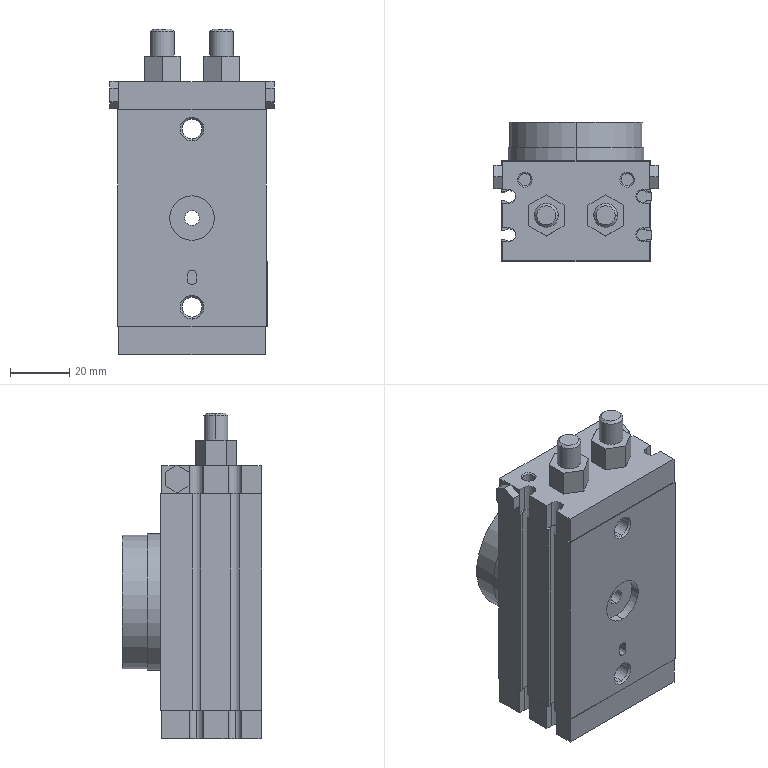Part | STEP file | Swing table MSQB10A | 2 solids | 264 faces | box 55.4 x 47 x 109.81 mm | volume 167301 mm3 | plane 129 | cylinder 91 | cone 44 | commonest cylinder face diameters 4.134 x28 4.6 x12 3 x9 4.2 x6 2.7 x4 4 x4